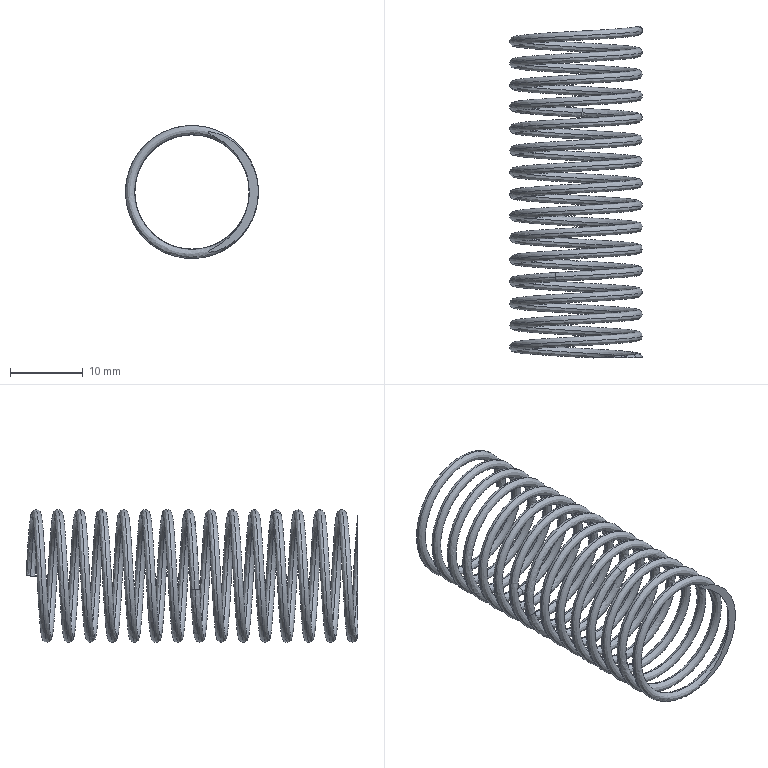Part | 1 solid | 11 faces | volume 980.273 mm3 | spline 9 | plane 2